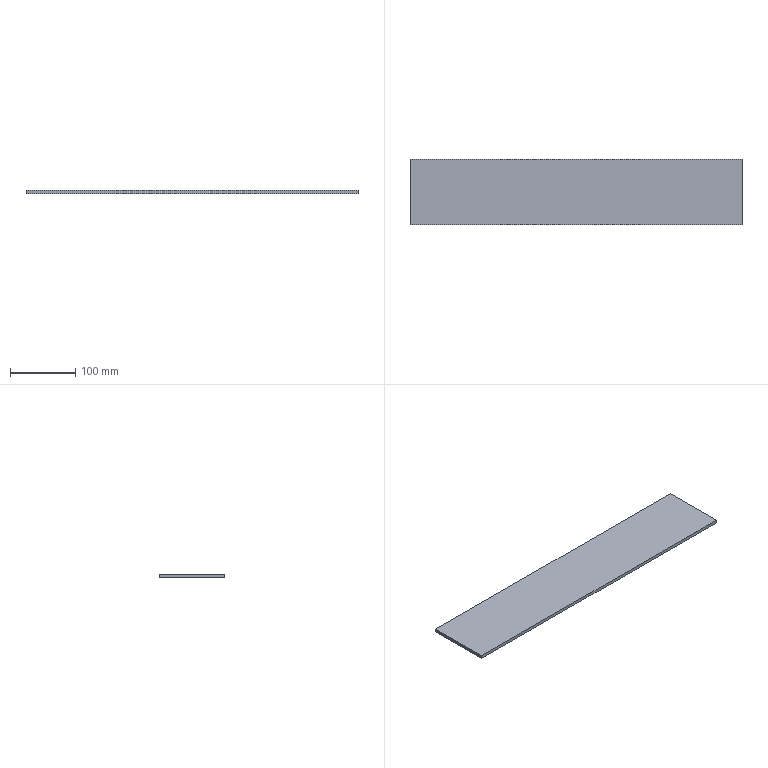Part | SolidWorks | features Extrusion 1 | 1 solid | 6 faces | box 510 x 100 x 5 mm | volume 255000 mm3 | plane 6
STEP:
#1=CARTESIAN_POINT('',(0.,100.,0.));
#2=VERTEX_POINT('',#1);
#3=CARTESIAN_POINT('',(0.,0.,0.));
#4=VERTEX_POINT('',#3);
#5=CARTESIAN_POINT('',(0.,0.,0.));
#6=DIRECTION('',(0.,-1.,0.));
#7=VECTOR('',#6,1000.);
#8=LINE('',#5,#7);
#9=EDGE_CURVE('',#2,#4,#8,.T.);
#10=ORIENTED_EDGE('',*,*,#9,.T.);
#11=CARTESIAN_POINT('',(0.,0.,5.));
#12=VERTEX_POINT('',#11);
#13=CARTESIAN_POINT('',(0.,0.,5.));
#14=DIRECTION('',(0.,0.,-1.));
#15=VECTOR('',#14,1000.);
#16=LINE('',#13,#15);
#17=EDGE_CURVE('',#12,#4,#16,.T.);
#18=ORIENTED_EDGE('',*,*,#17,.F.);
#19=CARTESIAN_POINT('',(0.,100.,5.));
#20=VERTEX_POINT('',#19);
#21=CARTESIAN_POINT('',(0.,0.,5.));
#22=DIRECTION('',(0.,-1.,0.));
#23=VECTOR('',#22,1000.);
#24=LINE('',#21,#23);
#25=EDGE_CURVE('',#20,#12,#24,.T.);
#26=ORIENTED_EDGE('',*,*,#25,.F.);
#27=CARTESIAN_POINT('',(0.,100.,5.));
#28=DIRECTION('',(0.,0.,-1.));
#29=VECTOR('',#28,1000.);
#30=LINE('',#27,#29);
#31=EDGE_CURVE('',#20,#2,#30,.T.);
#32=ORIENTED_EDGE('',*,*,#31,.T.);
#33=EDGE_LOOP('',(#10,#18,#26,#32));
#34=FACE_OUTER_BOUND('',#33,.T.);
#35=CARTESIAN_POINT('',(0.,0.,5.));
#36=DIRECTION('',(1.,0.,0.));
#37=DIRECTION('',(0.,0.,-1.));
#38=AXIS2_PLACEMENT_3D('',#35,#36,#37);
#39=PLANE('',#38);
#40=ADVANCED_FACE('',(#34),#39,.F.);
#41=CARTESIAN_POINT('',(510.,0.,0.));
#42=VERTEX_POINT('',#41);
#43=CARTESIAN_POINT('',(0.,0.,0.));
#44=DIRECTION('',(1.,0.,0.));
#45=VECTOR('',#44,1000.);
#46=LINE('',#43,#45);
#47=EDGE_CURVE('',#4,#42,#46,.T.);
#48=ORIENTED_EDGE('',*,*,#47,.T.);
#49=CARTESIAN_POINT('',(510.,0.,5.));
#50=VERTEX_POINT('',#49);
#51=CARTESIAN_POINT('',(510.,0.,5.));
#52=DIRECTION('',(0.,0.,-1.));
#53=VECTOR('',#52,1000.);
#54=LINE('',#51,#53);
#55=EDGE_CURVE('',#50,#42,#54,.T.);
#56=ORIENTED_EDGE('',*,*,#55,.F.);
#57=CARTESIAN_POINT('',(0.,0.,5.));
#58=DIRECTION('',(1.,0.,0.));
#59=VECTOR('',#58,1000.);
#60=LINE('',#57,#59);
#61=EDGE_CURVE('',#12,#50,#60,.T.);
#62=ORIENTED_EDGE('',*,*,#61,.F.);
#63=ORIENTED_EDGE('',*,*,#17,.T.);
#64=EDGE_LOOP('',(#48,#56,#62,#63));
#65=FACE_OUTER_BOUND('',#64,.T.);
#66=CARTESIAN_POINT('',(0.,0.,5.));
#67=DIRECTION('',(0.,1.,0.));
#68=DIRECTION('',(0.,0.,1.));
#69=AXIS2_PLACEMENT_3D('',#66,#67,#68);
#70=PLANE('',#69);
#71=ADVANCED_FACE('',(#65),#70,.F.);
#72=CARTESIAN_POINT('',(510.,100.,0.));
#73=VERTEX_POINT('',#72);
#74=CARTESIAN_POINT('',(510.,0.,0.));
#75=DIRECTION('',(0.,1.,0.));
#76=VECTOR('',#75,1000.);
#77=LINE('',#74,#76);
#78=EDGE_CURVE('',#42,#73,#77,.T.);
#79=ORIENTED_EDGE('',*,*,#78,.T.);
#80=CARTESIAN_POINT('',(510.,100.,5.));
#81=VERTEX_POINT('',#80);
#82=CARTESIAN_POINT('',(510.,100.,5.));
#83=DIRECTION('',(0.,0.,-1.));
#84=VECTOR('',#83,1000.);
#85=LINE('',#82,#84);
#86=EDGE_CURVE('',#81,#73,#85,.T.);
#87=ORIENTED_EDGE('',*,*,#86,.F.);
#88=CARTESIAN_POINT('',(510.,0.,5.));
#89=DIRECTION('',(0.,1.,0.));
#90=VECTOR('',#89,1000.);
#91=LINE('',#88,#90);
#92=EDGE_CURVE('',#50,#81,#91,.T.);
#93=ORIENTED_EDGE('',*,*,#92,.F.);
#94=ORIENTED_EDGE('',*,*,#55,.T.);
#95=EDGE_LOOP('',(#79,#87,#93,#94));
#96=FACE_OUTER_BOUND('',#95,.T.);
#97=CARTESIAN_POINT('',(510.,0.,5.));
#98=DIRECTION('',(-1.,0.,0.));
#99=DIRECTION('',(0.,0.,1.));
#100=AXIS2_PLACEMENT_3D('',#97,#98,#99);
#101=PLANE('',#100);
#102=ADVANCED_FACE('',(#96),#101,.F.);
#103=CARTESIAN_POINT('',(0.,100.,0.));
#104=DIRECTION('',(-1.,0.,0.));
#105=VECTOR('',#104,1000.);
#106=LINE('',#103,#105);
#107=EDGE_CURVE('',#73,#2,#106,.T.);
#108=ORIENTED_EDGE('',*,*,#107,.T.);
#109=ORIENTED_EDGE('',*,*,#31,.F.);
#110=CARTESIAN_POINT('',(0.,100.,5.));
#111=DIRECTION('',(-1.,0.,0.));
#112=VECTOR('',#111,1000.);
#113=LINE('',#110,#112);
#114=EDGE_CURVE('',#81,#20,#113,.T.);
#115=ORIENTED_EDGE('',*,*,#114,.F.);
#116=ORIENTED_EDGE('',*,*,#86,.T.);
#117=EDGE_LOOP('',(#108,#109,#115,#116));
#118=FACE_OUTER_BOUND('',#117,.T.);
#119=CARTESIAN_POINT('',(0.,100.,5.));
#120=DIRECTION('',(0.,-1.,0.));
#121=DIRECTION('',(0.,0.,-1.));
#122=AXIS2_PLACEMENT_3D('',#119,#120,#121);
#123=PLANE('',#122);
#124=ADVANCED_FACE('',(#118),#123,.F.);
#125=ORIENTED_EDGE('',*,*,#25,.T.);
#126=ORIENTED_EDGE('',*,*,#61,.T.);
#127=ORIENTED_EDGE('',*,*,#92,.T.);
#128=ORIENTED_EDGE('',*,*,#114,.T.);
#129=EDGE_LOOP('',(#125,#126,#127,#128));
#130=FACE_OUTER_BOUND('',#129,.T.);
#131=CARTESIAN_POINT('',(0.,0.,5.));
#132=DIRECTION('',(0.,0.,-1.));
#133=DIRECTION('',(-1.,0.,0.));
#134=AXIS2_PLACEMENT_3D('',#131,#132,#133);
#135=PLANE('',#134);
#136=ADVANCED_FACE('',(#130),#135,.F.);
#137=ORIENTED_EDGE('',*,*,#9,.F.);
#138=ORIENTED_EDGE('',*,*,#107,.F.);
#139=ORIENTED_EDGE('',*,*,#78,.F.);
#140=ORIENTED_EDGE('',*,*,#47,.F.);
#141=EDGE_LOOP('',(#137,#138,#139,#140));
#142=FACE_OUTER_BOUND('',#141,.T.);
#143=CARTESIAN_POINT('',(0.,0.,0.));
#144=DIRECTION('',(0.,0.,-1.));
#145=DIRECTION('',(-1.,0.,0.));
#146=AXIS2_PLACEMENT_3D('',#143,#144,#145);
#147=PLANE('',#146);
#148=ADVANCED_FACE('',(#142),#147,.T.);
#149=CLOSED_SHELL('',(#40,#71,#102,#124,#136,#148));
#150=MANIFOLD_SOLID_BREP('',#149);
#151=CARTESIAN_POINT('',(0.,0.,0.));
#152=DIRECTION('',(0.,0.,1.));
#153=DIRECTION('',(1.,0.,0.));
#154=AXIS2_PLACEMENT_3D('',#151,#152,#153);
#155=(LENGTH_UNIT()NAMED_UNIT(*)SI_UNIT(.MILLI.,.METRE.));
#156=UNCERTAINTY_MEASURE_WITH_UNIT(LENGTH_MEASURE(0.00001),#155,'','');
#157=(NAMED_UNIT(*)PLANE_ANGLE_UNIT()SI_UNIT($,.RADIAN.));
#158=(NAMED_UNIT(*)SI_UNIT($,.STERADIAN.)SOLID_ANGLE_UNIT());
#159=(GEOMETRIC_REPRESENTATION_CONTEXT(3)GLOBAL_UNCERTAINTY_ASSIGNED_CONTEXT((#156))GLOBAL_UNIT_ASSIGNED_CONTEXT((#155,#157,#158))REPRESENTATION_CONTEXT('',''));
#160=ADVANCED_BREP_SHAPE_REPRESENTATION('',(#150,#154),#159);